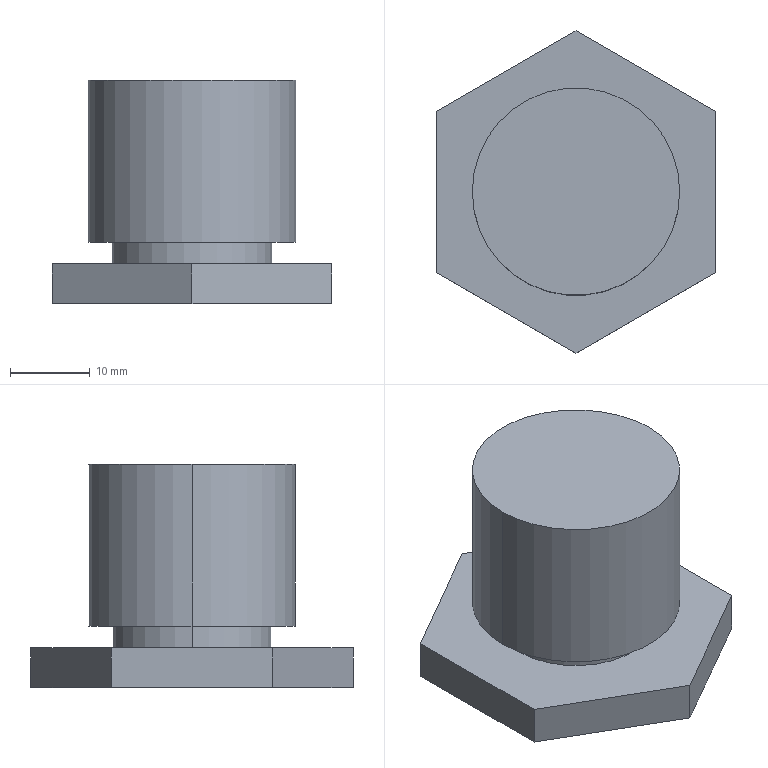Part | STEP file | Powder part sealing screw SGN-2-24 | 1 solid | 14 faces | box 35 x 40.415 x 28 mm | volume 16930 mm3 | plane 10 | cylinder 4 | commonest cylinder face diameters 20 x2 26 x2
STEP:
#1=CARTESIAN_POINT('',(0.,0.,0.));
#2=DIRECTION('',(0.,0.,1.));
#3=DIRECTION('',(1.,0.,0.));
#4=AXIS2_PLACEMENT_3D('',#1,#2,#3);
#5=CARTESIAN_POINT('',(13.,0.,23.));
#6=VERTEX_POINT('',#5);
#7=CARTESIAN_POINT('',(-13.,0.,23.));
#8=VERTEX_POINT('',#7);
#9=CARTESIAN_POINT('',(0.,0.,23.));
#10=DIRECTION('',(0.,0.,1.));
#11=DIRECTION('',(1.,0.,0.));
#12=AXIS2_PLACEMENT_3D('',#9,#10,#11);
#13=CIRCLE('',#12,13.);
#14=CARTESIAN_POINT('',(0.,0.,23.));
#15=DIRECTION('',(0.,0.,-1.));
#16=DIRECTION('',(-1.,0.,0.));
#17=AXIS2_PLACEMENT_3D('',#14,#15,#16);
#18=CYLINDRICAL_SURFACE('',#17,13.);
#19=CARTESIAN_POINT('',(3.142,0.));
#20=DIRECTION('',(-1.,0.));
#21=VECTOR('',#20,1.);
#22=LINE('',#19,#21);
#23=(GEOMETRIC_REPRESENTATION_CONTEXT(2)PARAMETRIC_REPRESENTATION_CONTEXT()REPRESENTATION_CONTEXT('',''));
#24=DEFINITIONAL_REPRESENTATION('',(#22),#23);
#25=PCURVE('',#18,#24);
#26=CARTESIAN_POINT('',(0.,0.,23.));
#27=DIRECTION('',(0.,0.,1.));
#28=DIRECTION('',(1.,0.,0.));
#29=AXIS2_PLACEMENT_3D('',#26,#27,#28);
#30=PLANE('',#29);
#31=CARTESIAN_POINT('',(0.,0.));
#32=DIRECTION('',(1.,0.));
#33=AXIS2_PLACEMENT_2D('',#31,#32);
#34=CIRCLE('',#33,13.);
#35=(GEOMETRIC_REPRESENTATION_CONTEXT(2)PARAMETRIC_REPRESENTATION_CONTEXT()REPRESENTATION_CONTEXT('',''));
#36=DEFINITIONAL_REPRESENTATION('',(#34),#35);
#37=PCURVE('',#30,#36);
#38=SURFACE_CURVE('',#13,(#25,#37),.PCURVE_S1.);
#39=EDGE_CURVE('',#6,#8,#38,.T.);
#40=ORIENTED_EDGE('',*,*,#39,.F.);
#41=CARTESIAN_POINT('',(13.,0.,2.7));
#42=VERTEX_POINT('',#41);
#43=CARTESIAN_POINT('',(13.,0.,23.));
#44=DIRECTION('',(0.,0.,-1.));
#45=VECTOR('',#44,1.);
#46=LINE('',#43,#45);
#47=CARTESIAN_POINT('',(3.142,0.));
#48=DIRECTION('',(0.,1.));
#49=VECTOR('',#48,1.);
#50=LINE('',#47,#49);
#51=(GEOMETRIC_REPRESENTATION_CONTEXT(2)PARAMETRIC_REPRESENTATION_CONTEXT()REPRESENTATION_CONTEXT('',''));
#52=DEFINITIONAL_REPRESENTATION('',(#50),#51);
#53=PCURVE('',#18,#52);
#54=CARTESIAN_POINT('',(0.,0.,23.));
#55=DIRECTION('',(0.,0.,-1.));
#56=DIRECTION('',(-1.,0.,0.));
#57=AXIS2_PLACEMENT_3D('',#54,#55,#56);
#58=CYLINDRICAL_SURFACE('',#57,13.);
#59=CARTESIAN_POINT('',(3.142,0.));
#60=DIRECTION('',(0.,1.));
#61=VECTOR('',#60,1.);
#62=LINE('',#59,#61);
#63=(GEOMETRIC_REPRESENTATION_CONTEXT(2)PARAMETRIC_REPRESENTATION_CONTEXT()REPRESENTATION_CONTEXT('',''));
#64=DEFINITIONAL_REPRESENTATION('',(#62),#63);
#65=PCURVE('',#58,#64);
#66=SURFACE_CURVE('',#46,(#53,#65),.PCURVE_S1.);
#67=EDGE_CURVE('',#6,#42,#66,.T.);
#68=ORIENTED_EDGE('',*,*,#67,.T.);
#69=CARTESIAN_POINT('',(-13.,0.,2.7));
#70=VERTEX_POINT('',#69);
#71=CARTESIAN_POINT('',(0.,0.,2.7));
#72=DIRECTION('',(0.,0.,1.));
#73=DIRECTION('',(1.,0.,0.));
#74=AXIS2_PLACEMENT_3D('',#71,#72,#73);
#75=CIRCLE('',#74,13.);
#76=CARTESIAN_POINT('',(3.142,20.3));
#77=DIRECTION('',(-1.,0.));
#78=VECTOR('',#77,1.);
#79=LINE('',#76,#78);
#80=(GEOMETRIC_REPRESENTATION_CONTEXT(2)PARAMETRIC_REPRESENTATION_CONTEXT()REPRESENTATION_CONTEXT('',''));
#81=DEFINITIONAL_REPRESENTATION('',(#79),#80);
#82=PCURVE('',#18,#81);
#83=CARTESIAN_POINT('',(0.,0.,2.7));
#84=DIRECTION('',(0.,0.,1.));
#85=DIRECTION('',(1.,0.,0.));
#86=AXIS2_PLACEMENT_3D('',#83,#84,#85);
#87=PLANE('',#86);
#88=CARTESIAN_POINT('',(0.,0.));
#89=DIRECTION('',(1.,0.));
#90=AXIS2_PLACEMENT_2D('',#88,#89);
#91=CIRCLE('',#90,13.);
#92=(GEOMETRIC_REPRESENTATION_CONTEXT(2)PARAMETRIC_REPRESENTATION_CONTEXT()REPRESENTATION_CONTEXT('',''));
#93=DEFINITIONAL_REPRESENTATION('',(#91),#92);
#94=PCURVE('',#87,#93);
#95=SURFACE_CURVE('',#75,(#82,#94),.PCURVE_S1.);
#96=EDGE_CURVE('',#42,#70,#95,.T.);
#97=ORIENTED_EDGE('',*,*,#96,.T.);
#98=CARTESIAN_POINT('',(-13.,0.,23.));
#99=DIRECTION('',(0.,0.,-1.));
#100=VECTOR('',#99,1.);
#101=LINE('',#98,#100);
#102=CARTESIAN_POINT('',(0.,0.));
#103=DIRECTION('',(0.,1.));
#104=VECTOR('',#103,1.);
#105=LINE('',#102,#104);
#106=(GEOMETRIC_REPRESENTATION_CONTEXT(2)PARAMETRIC_REPRESENTATION_CONTEXT()REPRESENTATION_CONTEXT('',''));
#107=DEFINITIONAL_REPRESENTATION('',(#105),#106);
#108=PCURVE('',#18,#107);
#109=CARTESIAN_POINT('',(6.283,0.));
#110=DIRECTION('',(0.,1.));
#111=VECTOR('',#110,1.);
#112=LINE('',#109,#111);
#113=(GEOMETRIC_REPRESENTATION_CONTEXT(2)PARAMETRIC_REPRESENTATION_CONTEXT()REPRESENTATION_CONTEXT('',''));
#114=DEFINITIONAL_REPRESENTATION('',(#112),#113);
#115=PCURVE('',#58,#114);
#116=SURFACE_CURVE('',#101,(#108,#115),.PCURVE_S1.);
#117=EDGE_CURVE('',#8,#70,#116,.T.);
#118=ORIENTED_EDGE('',*,*,#117,.F.);
#119=EDGE_LOOP('',(#40,#68,#97,#118));
#120=FACE_BOUND('',#119,.T.);
#121=ADVANCED_FACE('',(#120),#18,.T.);
#122=CARTESIAN_POINT('',(10.,0.,2.7));
#123=VERTEX_POINT('',#122);
#124=CARTESIAN_POINT('',(-10.,0.,2.7));
#125=VERTEX_POINT('',#124);
#126=CARTESIAN_POINT('',(0.,0.,2.7));
#127=DIRECTION('',(0.,0.,1.));
#128=DIRECTION('',(1.,0.,0.));
#129=AXIS2_PLACEMENT_3D('',#126,#127,#128);
#130=CIRCLE('',#129,10.);
#131=CARTESIAN_POINT('',(0.,0.,2.7));
#132=DIRECTION('',(0.,0.,-1.));
#133=DIRECTION('',(-1.,0.,0.));
#134=AXIS2_PLACEMENT_3D('',#131,#132,#133);
#135=CYLINDRICAL_SURFACE('',#134,10.);
#136=CARTESIAN_POINT('',(3.142,0.));
#137=DIRECTION('',(-1.,0.));
#138=VECTOR('',#137,1.);
#139=LINE('',#136,#138);
#140=(GEOMETRIC_REPRESENTATION_CONTEXT(2)PARAMETRIC_REPRESENTATION_CONTEXT()REPRESENTATION_CONTEXT('',''));
#141=DEFINITIONAL_REPRESENTATION('',(#139),#140);
#142=PCURVE('',#135,#141);
#143=CARTESIAN_POINT('',(0.,0.));
#144=DIRECTION('',(1.,0.));
#145=AXIS2_PLACEMENT_2D('',#143,#144);
#146=CIRCLE('',#145,10.);
#147=(GEOMETRIC_REPRESENTATION_CONTEXT(2)PARAMETRIC_REPRESENTATION_CONTEXT()REPRESENTATION_CONTEXT('',''));
#148=DEFINITIONAL_REPRESENTATION('',(#146),#147);
#149=PCURVE('',#87,#148);
#150=SURFACE_CURVE('',#130,(#142,#149),.PCURVE_S1.);
#151=EDGE_CURVE('',#123,#125,#150,.T.);
#152=ORIENTED_EDGE('',*,*,#151,.F.);
#153=CARTESIAN_POINT('',(10.,0.,0.));
#154=VERTEX_POINT('',#153);
#155=CARTESIAN_POINT('',(10.,0.,2.7));
#156=DIRECTION('',(0.,0.,-1.));
#157=VECTOR('',#156,1.);
#158=LINE('',#155,#157);
#159=CARTESIAN_POINT('',(3.142,0.));
#160=DIRECTION('',(0.,1.));
#161=VECTOR('',#160,1.);
#162=LINE('',#159,#161);
#163=(GEOMETRIC_REPRESENTATION_CONTEXT(2)PARAMETRIC_REPRESENTATION_CONTEXT()REPRESENTATION_CONTEXT('',''));
#164=DEFINITIONAL_REPRESENTATION('',(#162),#163);
#165=PCURVE('',#135,#164);
#166=CARTESIAN_POINT('',(0.,0.,2.7));
#167=DIRECTION('',(0.,0.,-1.));
#168=DIRECTION('',(-1.,0.,0.));
#169=AXIS2_PLACEMENT_3D('',#166,#167,#168);
#170=CYLINDRICAL_SURFACE('',#169,10.);
#171=CARTESIAN_POINT('',(3.142,0.));
#172=DIRECTION('',(0.,1.));
#173=VECTOR('',#172,1.);
#174=LINE('',#171,#173);
#175=(GEOMETRIC_REPRESENTATION_CONTEXT(2)PARAMETRIC_REPRESENTATION_CONTEXT()REPRESENTATION_CONTEXT('',''));
#176=DEFINITIONAL_REPRESENTATION('',(#174),#175);
#177=PCURVE('',#170,#176);
#178=SURFACE_CURVE('',#158,(#165,#177),.PCURVE_S1.);
#179=EDGE_CURVE('',#123,#154,#178,.T.);
#180=ORIENTED_EDGE('',*,*,#179,.T.);
#181=CARTESIAN_POINT('',(-10.,0.,0.));
#182=VERTEX_POINT('',#181);
#183=CARTESIAN_POINT('',(0.,0.,0.));
#184=DIRECTION('',(0.,0.,1.));
#185=DIRECTION('',(1.,0.,0.));
#186=AXIS2_PLACEMENT_3D('',#183,#184,#185);
#187=CIRCLE('',#186,10.);
#188=CARTESIAN_POINT('',(3.142,2.7));
#189=DIRECTION('',(-1.,0.));
#190=VECTOR('',#189,1.);
#191=LINE('',#188,#190);
#192=(GEOMETRIC_REPRESENTATION_CONTEXT(2)PARAMETRIC_REPRESENTATION_CONTEXT()REPRESENTATION_CONTEXT('',''));
#193=DEFINITIONAL_REPRESENTATION('',(#191),#192);
#194=PCURVE('',#135,#193);
#195=CARTESIAN_POINT('',(0.,0.,0.));
#196=DIRECTION('',(0.,0.,-1.));
#197=DIRECTION('',(-1.,0.,0.));
#198=AXIS2_PLACEMENT_3D('',#195,#196,#197);
#199=PLANE('',#198);
#200=CARTESIAN_POINT('',(-10.,0.));
#201=CARTESIAN_POINT('',(-10.,17.321));
#202=CARTESIAN_POINT('',(5.,8.66));
#203=CARTESIAN_POINT('',(20.,0.));
#204=CARTESIAN_POINT('',(5.,-8.66));
#205=CARTESIAN_POINT('',(-10.,-17.321));
#206=CARTESIAN_POINT('',(-10.,0.));
#207=(BOUNDED_CURVE()B_SPLINE_CURVE(2,(#200,#201,#202,#203,#204,#205,#206),.UNSPECIFIED.,.T.,.F.)B_SPLINE_CURVE_WITH_KNOTS((1,2,2,2,2,1),(-2.094,0.,2.094,4.189,6.283,8.378),.UNSPECIFIED.)CURVE()GEOMETRIC_REPRESENTATION_ITEM()RATIONAL_B_SPLINE_CURVE((1.,0.5,1.,0.5,1.,0.5,1.))REPRESENTATION_ITEM(''));
#208=(GEOMETRIC_REPRESENTATION_CONTEXT(2)PARAMETRIC_REPRESENTATION_CONTEXT()REPRESENTATION_CONTEXT('',''));
#209=DEFINITIONAL_REPRESENTATION('',(#207),#208);
#210=PCURVE('',#199,#209);
#211=SURFACE_CURVE('',#187,(#194,#210),.PCURVE_S1.);
#212=EDGE_CURVE('',#154,#182,#211,.T.);
#213=ORIENTED_EDGE('',*,*,#212,.T.);
#214=CARTESIAN_POINT('',(-10.,0.,2.7));
#215=DIRECTION('',(0.,0.,-1.));
#216=VECTOR('',#215,1.);
#217=LINE('',#214,#216);
#218=CARTESIAN_POINT('',(0.,0.));
#219=DIRECTION('',(0.,1.));
#220=VECTOR('',#219,1.);
#221=LINE('',#218,#220);
#222=(GEOMETRIC_REPRESENTATION_CONTEXT(2)PARAMETRIC_REPRESENTATION_CONTEXT()REPRESENTATION_CONTEXT('',''));
#223=DEFINITIONAL_REPRESENTATION('',(#221),#222);
#224=PCURVE('',#135,#223);
#225=CARTESIAN_POINT('',(6.283,0.));
#226=DIRECTION('',(0.,1.));
#227=VECTOR('',#226,1.);
#228=LINE('',#225,#227);
#229=(GEOMETRIC_REPRESENTATION_CONTEXT(2)PARAMETRIC_REPRESENTATION_CONTEXT()REPRESENTATION_CONTEXT('',''));
#230=DEFINITIONAL_REPRESENTATION('',(#228),#229);
#231=PCURVE('',#170,#230);
#232=SURFACE_CURVE('',#217,(#224,#231),.PCURVE_S1.);
#233=EDGE_CURVE('',#125,#182,#232,.T.);
#234=ORIENTED_EDGE('',*,*,#233,.F.);
#235=EDGE_LOOP('',(#152,#180,#213,#234));
#236=FACE_BOUND('',#235,.T.);
#237=ADVANCED_FACE('',(#236),#135,.T.);
#238=CARTESIAN_POINT('',(-17.5,10.104,0.));
#239=VERTEX_POINT('',#238);
#240=CARTESIAN_POINT('',(0.,20.207,0.));
#241=VERTEX_POINT('',#240);
#242=CARTESIAN_POINT('',(-17.5,10.104,0.));
#243=DIRECTION('',(0.866,0.5,0.));
#244=VECTOR('',#243,1.);
#245=LINE('',#242,#244);
#246=CARTESIAN_POINT('',(-17.5,10.104,-5.));
#247=DIRECTION('',(0.5,-0.866,0.));
#248=DIRECTION('',(0.866,0.5,0.));
#249=AXIS2_PLACEMENT_3D('',#246,#247,#248);
#250=PLANE('',#249);
#251=CARTESIAN_POINT('',(0.,5.));
#252=DIRECTION('',(1.,0.));
#253=VECTOR('',#252,1.);
#254=LINE('',#251,#253);
#255=(GEOMETRIC_REPRESENTATION_CONTEXT(2)PARAMETRIC_REPRESENTATION_CONTEXT()REPRESENTATION_CONTEXT('',''));
#256=DEFINITIONAL_REPRESENTATION('',(#254),#255);
#257=PCURVE('',#250,#256);
#258=CARTESIAN_POINT('',(17.5,10.104));
#259=DIRECTION('',(-0.866,0.5));
#260=VECTOR('',#259,1.);
#261=LINE('',#258,#260);
#262=(GEOMETRIC_REPRESENTATION_CONTEXT(2)PARAMETRIC_REPRESENTATION_CONTEXT()REPRESENTATION_CONTEXT('',''));
#263=DEFINITIONAL_REPRESENTATION('',(#261),#262);
#264=PCURVE('',#199,#263);
#265=SURFACE_CURVE('',#245,(#257,#264),.PCURVE_S1.);
#266=EDGE_CURVE('',#239,#241,#265,.T.);
#267=ORIENTED_EDGE('',*,*,#266,.T.);
#268=CARTESIAN_POINT('',(0.,20.207,-5.));
#269=VERTEX_POINT('',#268);
#270=CARTESIAN_POINT('',(0.,20.207,-5.));
#271=DIRECTION('',(0.,0.,1.));
#272=VECTOR('',#271,1.);
#273=LINE('',#270,#272);
#274=CARTESIAN_POINT('',(20.207,0.));
#275=DIRECTION('',(0.,1.));
#276=VECTOR('',#275,1.);
#277=LINE('',#274,#276);
#278=(GEOMETRIC_REPRESENTATION_CONTEXT(2)PARAMETRIC_REPRESENTATION_CONTEXT()REPRESENTATION_CONTEXT('',''));
#279=DEFINITIONAL_REPRESENTATION('',(#277),#278);
#280=PCURVE('',#250,#279);
#281=CARTESIAN_POINT('',(0.,20.207,-5.));
#282=DIRECTION('',(-0.5,-0.866,0.));
#283=DIRECTION('',(0.866,-0.5,0.));
#284=AXIS2_PLACEMENT_3D('',#281,#282,#283);
#285=PLANE('',#284);
#286=CARTESIAN_POINT('',(0.,0.));
#287=DIRECTION('',(0.,1.));
#288=VECTOR('',#287,1.);
#289=LINE('',#286,#288);
#290=(GEOMETRIC_REPRESENTATION_CONTEXT(2)PARAMETRIC_REPRESENTATION_CONTEXT()REPRESENTATION_CONTEXT('',''));
#291=DEFINITIONAL_REPRESENTATION('',(#289),#290);
#292=PCURVE('',#285,#291);
#293=SURFACE_CURVE('',#273,(#280,#292),.PCURVE_S1.);
#294=EDGE_CURVE('',#269,#241,#293,.T.);
#295=ORIENTED_EDGE('',*,*,#294,.F.);
#296=CARTESIAN_POINT('',(-17.5,10.104,-5.));
#297=VERTEX_POINT('',#296);
#298=CARTESIAN_POINT('',(-17.5,10.104,-5.));
#299=DIRECTION('',(0.866,0.5,0.));
#300=VECTOR('',#299,1.);
#301=LINE('',#298,#300);
#302=CARTESIAN_POINT('',(0.,0.));
#303=DIRECTION('',(1.,0.));
#304=VECTOR('',#303,1.);
#305=LINE('',#302,#304);
#306=(GEOMETRIC_REPRESENTATION_CONTEXT(2)PARAMETRIC_REPRESENTATION_CONTEXT()REPRESENTATION_CONTEXT('',''));
#307=DEFINITIONAL_REPRESENTATION('',(#305),#306);
#308=PCURVE('',#250,#307);
#309=CARTESIAN_POINT('',(0.,0.,-5.));
#310=DIRECTION('',(0.,0.,-1.));
#311=DIRECTION('',(-1.,0.,0.));
#312=AXIS2_PLACEMENT_3D('',#309,#310,#311);
#313=PLANE('',#312);
#314=CARTESIAN_POINT('',(17.5,10.104));
#315=DIRECTION('',(-0.866,0.5));
#316=VECTOR('',#315,1.);
#317=LINE('',#314,#316);
#318=(GEOMETRIC_REPRESENTATION_CONTEXT(2)PARAMETRIC_REPRESENTATION_CONTEXT()REPRESENTATION_CONTEXT('',''));
#319=DEFINITIONAL_REPRESENTATION('',(#317),#318);
#320=PCURVE('',#313,#319);
#321=SURFACE_CURVE('',#301,(#308,#320),.PCURVE_S1.);
#322=EDGE_CURVE('',#297,#269,#321,.T.);
#323=ORIENTED_EDGE('',*,*,#322,.F.);
#324=CARTESIAN_POINT('',(-17.5,10.104,-5.));
#325=DIRECTION('',(0.,0.,1.));
#326=VECTOR('',#325,1.);
#327=LINE('',#324,#326);
#328=CARTESIAN_POINT('',(0.,0.));
#329=DIRECTION('',(0.,1.));
#330=VECTOR('',#329,1.);
#331=LINE('',#328,#330);
#332=(GEOMETRIC_REPRESENTATION_CONTEXT(2)PARAMETRIC_REPRESENTATION_CONTEXT()REPRESENTATION_CONTEXT('',''));
#333=DEFINITIONAL_REPRESENTATION('',(#331),#332);
#334=PCURVE('',#250,#333);
#335=CARTESIAN_POINT('',(-17.5,-10.104,-5.));
#336=DIRECTION('',(1.,0.,0.));
#337=DIRECTION('',(0.,1.,0.));
#338=AXIS2_PLACEMENT_3D('',#335,#336,#337);
#339=PLANE('',#338);
#340=CARTESIAN_POINT('',(20.207,0.));
#341=DIRECTION('',(0.,1.));
#342=VECTOR('',#341,1.);
#343=LINE('',#340,#342);
#344=(GEOMETRIC_REPRESENTATION_CONTEXT(2)PARAMETRIC_REPRESENTATION_CONTEXT()REPRESENTATION_CONTEXT('',''));
#345=DEFINITIONAL_REPRESENTATION('',(#343),#344);
#346=PCURVE('',#339,#345);
#347=SURFACE_CURVE('',#327,(#334,#346),.PCURVE_S1.);
#348=EDGE_CURVE('',#297,#239,#347,.T.);
#349=ORIENTED_EDGE('',*,*,#348,.T.);
#350=EDGE_LOOP('',(#267,#295,#323,#349));
#351=FACE_BOUND('',#350,.T.);
#352=ADVANCED_FACE('',(#351),#250,.F.);
#353=CARTESIAN_POINT('',(17.5,10.104,0.));
#354=VERTEX_POINT('',#353);
#355=CARTESIAN_POINT('',(0.,20.207,0.));
#356=DIRECTION('',(0.866,-0.5,0.));
#357=VECTOR('',#356,1.);
#358=LINE('',#355,#357);
#359=CARTESIAN_POINT('',(0.,5.));
#360=DIRECTION('',(1.,0.));
#361=VECTOR('',#360,1.);
#362=LINE('',#359,#361);
#363=(GEOMETRIC_REPRESENTATION_CONTEXT(2)PARAMETRIC_REPRESENTATION_CONTEXT()REPRESENTATION_CONTEXT('',''));
#364=DEFINITIONAL_REPRESENTATION('',(#362),#363);
#365=PCURVE('',#285,#364);
#366=CARTESIAN_POINT('',(0.,20.207));
#367=DIRECTION('',(-0.866,-0.5));
#368=VECTOR('',#367,1.);
#369=LINE('',#366,#368);
#370=(GEOMETRIC_REPRESENTATION_CONTEXT(2)PARAMETRIC_REPRESENTATION_CONTEXT()REPRESENTATION_CONTEXT('',''));
#371=DEFINITIONAL_REPRESENTATION('',(#369),#370);
#372=PCURVE('',#199,#371);
#373=SURFACE_CURVE('',#358,(#365,#372),.PCURVE_S1.);
#374=EDGE_CURVE('',#241,#354,#373,.T.);
#375=ORIENTED_EDGE('',*,*,#374,.T.);
#376=CARTESIAN_POINT('',(17.5,10.104,-5.));
#377=VERTEX_POINT('',#376);
#378=CARTESIAN_POINT('',(17.5,10.104,-5.));
#379=DIRECTION('',(0.,0.,1.));
#380=VECTOR('',#379,1.);
#381=LINE('',#378,#380);
#382=CARTESIAN_POINT('',(20.207,0.));
#383=DIRECTION('',(0.,1.));
#384=VECTOR('',#383,1.);
#385=LINE('',#382,#384);
#386=(GEOMETRIC_REPRESENTATION_CONTEXT(2)PARAMETRIC_REPRESENTATION_CONTEXT()REPRESENTATION_CONTEXT('',''));
#387=DEFINITIONAL_REPRESENTATION('',(#385),#386);
#388=PCURVE('',#285,#387);
#389=CARTESIAN_POINT('',(17.5,10.104,-5.));
#390=DIRECTION('',(-1.,0.,0.));
#391=DIRECTION('',(0.,-1.,0.));
#392=AXIS2_PLACEMENT_3D('',#389,#390,#391);
#393=PLANE('',#392);
#394=CARTESIAN_POINT('',(0.,0.));
#395=DIRECTION('',(0.,1.));
#396=VECTOR('',#395,1.);
#397=LINE('',#394,#396);
#398=(GEOMETRIC_REPRESENTATION_CONTEXT(2)PARAMETRIC_REPRESENTATION_CONTEXT()REPRESENTATION_CONTEXT('',''));
#399=DEFINITIONAL_REPRESENTATION('',(#397),#398);
#400=PCURVE('',#393,#399);
#401=SURFACE_CURVE('',#381,(#388,#400),.PCURVE_S1.);
#402=EDGE_CURVE('',#377,#354,#401,.T.);
#403=ORIENTED_EDGE('',*,*,#402,.F.);
#404=CARTESIAN_POINT('',(0.,20.207,-5.));
#405=DIRECTION('',(0.866,-0.5,0.));
#406=VECTOR('',#405,1.);
#407=LINE('',#404,#406);
#408=CARTESIAN_POINT('',(0.,0.));
#409=DIRECTION('',(1.,0.));
#410=VECTOR('',#409,1.);
#411=LINE('',#408,#410);
#412=(GEOMETRIC_REPRESENTATION_CONTEXT(2)PARAMETRIC_REPRESENTATION_CONTEXT()REPRESENTATION_CONTEXT('',''));
#413=DEFINITIONAL_REPRESENTATION('',(#411),#412);
#414=PCURVE('',#285,#413);
#415=CARTESIAN_POINT('',(0.,20.207));
#416=DIRECTION('',(-0.866,-0.5));
#417=VECTOR('',#416,1.);
#418=LINE('',#415,#417);
#419=(GEOMETRIC_REPRESENTATION_CONTEXT(2)PARAMETRIC_REPRESENTATION_CONTEXT()REPRESENTATION_CONTEXT('',''));
#420=DEFINITIONAL_REPRESENTATION('',(#418),#419);
#421=PCURVE('',#313,#420);
#422=SURFACE_CURVE('',#407,(#414,#421),.PCURVE_S1.);
#423=EDGE_CURVE('',#269,#377,#422,.T.);
#424=ORIENTED_EDGE('',*,*,#423,.F.);
#425=ORIENTED_EDGE('',*,*,#294,.T.);
#426=EDGE_LOOP('',(#375,#403,#424,#425));
#427=FACE_BOUND('',#426,.T.);
#428=ADVANCED_FACE('',(#427),#285,.F.);
#429=CARTESIAN_POINT('',(17.5,-10.104,0.));
#430=VERTEX_POINT('',#429);
#431=CARTESIAN_POINT('',(17.5,10.104,0.));
#432=DIRECTION('',(0.,-1.,0.));
#433=VECTOR('',#432,1.);
#434=LINE('',#431,#433);
#435=CARTESIAN_POINT('',(0.,5.));
#436=DIRECTION('',(1.,0.));
#437=VECTOR('',#436,1.);
#438=LINE('',#435,#437);
#439=(GEOMETRIC_REPRESENTATION_CONTEXT(2)PARAMETRIC_REPRESENTATION_CONTEXT()REPRESENTATION_CONTEXT('',''));
#440=DEFINITIONAL_REPRESENTATION('',(#438),#439);
#441=PCURVE('',#393,#440);
#442=CARTESIAN_POINT('',(-17.5,10.104));
#443=DIRECTION('',(0.,-1.));
#444=VECTOR('',#443,1.);
#445=LINE('',#442,#444);
#446=(GEOMETRIC_REPRESENTATION_CONTEXT(2)PARAMETRIC_REPRESENTATION_CONTEXT()REPRESENTATION_CONTEXT('',''));
#447=DEFINITIONAL_REPRESENTATION('',(#445),#446);
#448=PCURVE('',#199,#447);
#449=SURFACE_CURVE('',#434,(#441,#448),.PCURVE_S1.);
#450=EDGE_CURVE('',#354,#430,#449,.T.);
#451=ORIENTED_EDGE('',*,*,#450,.T.);
#452=CARTESIAN_POINT('',(17.5,-10.104,-5.));
#453=VERTEX_POINT('',#452);
#454=CARTESIAN_POINT('',(17.5,-10.104,-5.));
#455=DIRECTION('',(0.,0.,1.));
#456=VECTOR('',#455,1.);
#457=LINE('',#454,#456);
#458=CARTESIAN_POINT('',(20.207,0.));
#459=DIRECTION('',(0.,1.));
#460=VECTOR('',#459,1.);
#461=LINE('',#458,#460);
#462=(GEOMETRIC_REPRESENTATION_CONTEXT(2)PARAMETRIC_REPRESENTATION_CONTEXT()REPRESENTATION_CONTEXT('',''));
#463=DEFINITIONAL_REPRESENTATION('',(#461),#462);
#464=PCURVE('',#393,#463);
#465=CARTESIAN_POINT('',(17.5,-10.104,-5.));
#466=DIRECTION('',(-0.5,0.866,0.));
#467=DIRECTION('',(-0.866,-0.5,0.));
#468=AXIS2_PLACEMENT_3D('',#465,#466,#467);
#469=PLANE('',#468);
#470=CARTESIAN_POINT('',(0.,0.));
#471=DIRECTION('',(0.,1.));
#472=VECTOR('',#471,1.);
#473=LINE('',#470,#472);
#474=(GEOMETRIC_REPRESENTATION_CONTEXT(2)PARAMETRIC_REPRESENTATION_CONTEXT()REPRESENTATION_CONTEXT('',''));
#475=DEFINITIONAL_REPRESENTATION('',(#473),#474);
#476=PCURVE('',#469,#475);
#477=SURFACE_CURVE('',#457,(#464,#476),.PCURVE_S1.);
#478=EDGE_CURVE('',#453,#430,#477,.T.);
#479=ORIENTED_EDGE('',*,*,#478,.F.);
#480=CARTESIAN_POINT('',(17.5,10.104,-5.));
#481=DIRECTION('',(0.,-1.,0.));
#482=VECTOR('',#481,1.);
#483=LINE('',#480,#482);
#484=CARTESIAN_POINT('',(0.,0.));
#485=DIRECTION('',(1.,0.));
#486=VECTOR('',#485,1.);
#487=LINE('',#484,#486);
#488=(GEOMETRIC_REPRESENTATION_CONTEXT(2)PARAMETRIC_REPRESENTATION_CONTEXT()REPRESENTATION_CONTEXT('',''));
#489=DEFINITIONAL_REPRESENTATION('',(#487),#488);
#490=PCURVE('',#393,#489);
#491=CARTESIAN_POINT('',(-17.5,10.104));
#492=DIRECTION('',(0.,-1.));
#493=VECTOR('',#492,1.);
#494=LINE('',#491,#493);
#495=(GEOMETRIC_REPRESENTATION_CONTEXT(2)PARAMETRIC_REPRESENTATION_CONTEXT()REPRESENTATION_CONTEXT('',''));
#496=DEFINITIONAL_REPRESENTATION('',(#494),#495);
#497=PCURVE('',#313,#496);
#498=SURFACE_CURVE('',#483,(#490,#497),.PCURVE_S1.);
#499=EDGE_CURVE('',#377,#453,#498,.T.);
#500=ORIENTED_EDGE('',*,*,#499,.F.);
#501=ORIENTED_EDGE('',*,*,#402,.T.);
#502=EDGE_LOOP('',(#451,#479,#500,#501));
#503=FACE_BOUND('',#502,.T.);
#504=ADVANCED_FACE('',(#503),#393,.F.);
#505=CARTESIAN_POINT('',(0.,-20.207,0.));
#506=VERTEX_POINT('',#505);
#507=CARTESIAN_POINT('',(17.5,-10.104,0.));
#508=DIRECTION('',(-0.866,-0.5,0.));
#509=VECTOR('',#508,1.);
#510=LINE('',#507,#509);
#511=CARTESIAN_POINT('',(0.,5.));
#512=DIRECTION('',(1.,0.));
#513=VECTOR('',#512,1.);
#514=LINE('',#511,#513);
#515=(GEOMETRIC_REPRESENTATION_CONTEXT(2)PARAMETRIC_REPRESENTATION_CONTEXT()REPRESENTATION_CONTEXT('',''));
#516=DEFINITIONAL_REPRESENTATION('',(#514),#515);
#517=PCURVE('',#469,#516);
#518=CARTESIAN_POINT('',(-17.5,-10.104));
#519=DIRECTION('',(0.866,-0.5));
#520=VECTOR('',#519,1.);
#521=LINE('',#518,#520);
#522=(GEOMETRIC_REPRESENTATION_CONTEXT(2)PARAMETRIC_REPRESENTATION_CONTEXT()REPRESENTATION_CONTEXT('',''));
#523=DEFINITIONAL_REPRESENTATION('',(#521),#522);
#524=PCURVE('',#199,#523);
#525=SURFACE_CURVE('',#510,(#517,#524),.PCURVE_S1.);
#526=EDGE_CURVE('',#430,#506,#525,.T.);
#527=ORIENTED_EDGE('',*,*,#526,.T.);
#528=CARTESIAN_POINT('',(0.,-20.207,-5.));
#529=VERTEX_POINT('',#528);
#530=CARTESIAN_POINT('',(0.,-20.207,-5.));
#531=DIRECTION('',(0.,0.,1.));
#532=VECTOR('',#531,1.);
#533=LINE('',#530,#532);
#534=CARTESIAN_POINT('',(20.207,0.));
#535=DIRECTION('',(0.,1.));
#536=VECTOR('',#535,1.);
#537=LINE('',#534,#536);
#538=(GEOMETRIC_REPRESENTATION_CONTEXT(2)PARAMETRIC_REPRESENTATION_CONTEXT()REPRESENTATION_CONTEXT('',''));
#539=DEFINITIONAL_REPRESENTATION('',(#537),#538);
#540=PCURVE('',#469,#539);
#541=CARTESIAN_POINT('',(0.,-20.207,-5.));
#542=DIRECTION('',(0.5,0.866,0.));
#543=DIRECTION('',(-0.866,0.5,0.));
#544=AXIS2_PLACEMENT_3D('',#541,#542,#543);
#545=PLANE('',#544);
#546=CARTESIAN_POINT('',(0.,0.));
#547=DIRECTION('',(0.,1.));
#548=VECTOR('',#547,1.);
#549=LINE('',#546,#548);
#550=(GEOMETRIC_REPRESENTATION_CONTEXT(2)PARAMETRIC_REPRESENTATION_CONTEXT()REPRESENTATION_CONTEXT('',''));
#551=DEFINITIONAL_REPRESENTATION('',(#549),#550);
#552=PCURVE('',#545,#551);
#553=SURFACE_CURVE('',#533,(#540,#552),.PCURVE_S1.);
#554=EDGE_CURVE('',#529,#506,#553,.T.);
#555=ORIENTED_EDGE('',*,*,#554,.F.);
#556=CARTESIAN_POINT('',(17.5,-10.104,-5.));
#557=DIRECTION('',(-0.866,-0.5,0.));
#558=VECTOR('',#557,1.);
#559=LINE('',#556,#558);
#560=CARTESIAN_POINT('',(0.,0.));
#561=DIRECTION('',(1.,0.));
#562=VECTOR('',#561,1.);
#563=LINE('',#560,#562);
#564=(GEOMETRIC_REPRESENTATION_CONTEXT(2)PARAMETRIC_REPRESENTATION_CONTEXT()REPRESENTATION_CONTEXT('',''));
#565=DEFINITIONAL_REPRESENTATION('',(#563),#564);
#566=PCURVE('',#469,#565);
#567=CARTESIAN_POINT('',(-17.5,-10.104));
#568=DIRECTION('',(0.866,-0.5));
#569=VECTOR('',#568,1.);
#570=LINE('',#567,#569);
#571=(GEOMETRIC_REPRESENTATION_CONTEXT(2)PARAMETRIC_REPRESENTATION_CONTEXT()REPRESENTATION_CONTEXT('',''));
#572=DEFINITIONAL_REPRESENTATION('',(#570),#571);
#573=PCURVE('',#313,#572);
#574=SURFACE_CURVE('',#559,(#566,#573),.PCURVE_S1.);
#575=EDGE_CURVE('',#453,#529,#574,.T.);
#576=ORIENTED_EDGE('',*,*,#575,.F.);
#577=ORIENTED_EDGE('',*,*,#478,.T.);
#578=EDGE_LOOP('',(#527,#555,#576,#577));
#579=FACE_BOUND('',#578,.T.);
#580=ADVANCED_FACE('',(#579),#469,.F.);
#581=CARTESIAN_POINT('',(-17.5,-10.104,0.));
#582=VERTEX_POINT('',#581);
#583=CARTESIAN_POINT('',(0.,-20.207,0.));
#584=DIRECTION('',(-0.866,0.5,0.));
#585=VECTOR('',#584,1.);
#586=LINE('',#583,#585);
#587=CARTESIAN_POINT('',(0.,5.));
#588=DIRECTION('',(1.,0.));
#589=VECTOR('',#588,1.);
#590=LINE('',#587,#589);
#591=(GEOMETRIC_REPRESENTATION_CONTEXT(2)PARAMETRIC_REPRESENTATION_CONTEXT()REPRESENTATION_CONTEXT('',''));
#592=DEFINITIONAL_REPRESENTATION('',(#590),#591);
#593=PCURVE('',#545,#592);
#594=CARTESIAN_POINT('',(0.,-20.207));
#595=DIRECTION('',(0.866,0.5));
#596=VECTOR('',#595,1.);
#597=LINE('',#594,#596);
#598=(GEOMETRIC_REPRESENTATION_CONTEXT(2)PARAMETRIC_REPRESENTATION_CONTEXT()REPRESENTATION_CONTEXT('',''));
#599=DEFINITIONAL_REPRESENTATION('',(#597),#598);
#600=PCURVE('',#199,#599);
#601=SURFACE_CURVE('',#586,(#593,#600),.PCURVE_S1.);
#602=EDGE_CURVE('',#506,#582,#601,.T.);
#603=ORIENTED_EDGE('',*,*,#602,.T.);
#604=CARTESIAN_POINT('',(-17.5,-10.104,-5.));
#605=VERTEX_POINT('',#604);
#606=CARTESIAN_POINT('',(-17.5,-10.104,-5.));
#607=DIRECTION('',(0.,0.,1.));
#608=VECTOR('',#607,1.);
#609=LINE('',#606,#608);
#610=CARTESIAN_POINT('',(20.207,0.));
#611=DIRECTION('',(0.,1.));
#612=VECTOR('',#611,1.);
#613=LINE('',#610,#612);
#614=(GEOMETRIC_REPRESENTATION_CONTEXT(2)PARAMETRIC_REPRESENTATION_CONTEXT()REPRESENTATION_CONTEXT('',''));
#615=DEFINITIONAL_REPRESENTATION('',(#613),#614);
#616=PCURVE('',#545,#615);
#617=CARTESIAN_POINT('',(0.,0.));
#618=DIRECTION('',(0.,1.));
#619=VECTOR('',#618,1.);
#620=LINE('',#617,#619);
#621=(GEOMETRIC_REPRESENTATION_CONTEXT(2)PARAMETRIC_REPRESENTATION_CONTEXT()REPRESENTATION_CONTEXT('',''));
#622=DEFINITIONAL_REPRESENTATION('',(#620),#621);
#623=PCURVE('',#339,#622);
#624=SURFACE_CURVE('',#609,(#616,#623),.PCURVE_S1.);
#625=EDGE_CURVE('',#605,#582,#624,.T.);
#626=ORIENTED_EDGE('',*,*,#625,.F.);
#627=CARTESIAN_POINT('',(0.,-20.207,-5.));
#628=DIRECTION('',(-0.866,0.5,0.));
#629=VECTOR('',#628,1.);
#630=LINE('',#627,#629);
#631=CARTESIAN_POINT('',(0.,0.));
#632=DIRECTION('',(1.,0.));
#633=VECTOR('',#632,1.);
#634=LINE('',#631,#633);
#635=(GEOMETRIC_REPRESENTATION_CONTEXT(2)PARAMETRIC_REPRESENTATION_CONTEXT()REPRESENTATION_CONTEXT('',''));
#636=DEFINITIONAL_REPRESENTATION('',(#634),#635);
#637=PCURVE('',#545,#636);
#638=CARTESIAN_POINT('',(0.,-20.207));
#639=DIRECTION('',(0.866,0.5));
#640=VECTOR('',#639,1.);
#641=LINE('',#638,#640);
#642=(GEOMETRIC_REPRESENTATION_CONTEXT(2)PARAMETRIC_REPRESENTATION_CONTEXT()REPRESENTATION_CONTEXT('',''));
#643=DEFINITIONAL_REPRESENTATION('',(#641),#642);
#644=PCURVE('',#313,#643);
#645=SURFACE_CURVE('',#630,(#637,#644),.PCURVE_S1.);
#646=EDGE_CURVE('',#529,#605,#645,.T.);
#647=ORIENTED_EDGE('',*,*,#646,.F.);
#648=ORIENTED_EDGE('',*,*,#554,.T.);
#649=EDGE_LOOP('',(#603,#626,#647,#648));
#650=FACE_BOUND('',#649,.T.);
#651=ADVANCED_FACE('',(#650),#545,.F.);
#652=CARTESIAN_POINT('',(-17.5,-10.104,0.));
#653=DIRECTION('',(0.,1.,0.));
#654=VECTOR('',#653,1.);
#655=LINE('',#652,#654);
#656=CARTESIAN_POINT('',(0.,5.));
#657=DIRECTION('',(1.,0.));
#658=VECTOR('',#657,1.);
#659=LINE('',#656,#658);
#660=(GEOMETRIC_REPRESENTATION_CONTEXT(2)PARAMETRIC_REPRESENTATION_CONTEXT()REPRESENTATION_CONTEXT('',''));
#661=DEFINITIONAL_REPRESENTATION('',(#659),#660);
#662=PCURVE('',#339,#661);
#663=CARTESIAN_POINT('',(17.5,-10.104));
#664=DIRECTION('',(0.,1.));
#665=VECTOR('',#664,1.);
#666=LINE('',#663,#665);
#667=(GEOMETRIC_REPRESENTATION_CONTEXT(2)PARAMETRIC_REPRESENTATION_CONTEXT()REPRESENTATION_CONTEXT('',''));
#668=DEFINITIONAL_REPRESENTATION('',(#666),#667);
#669=PCURVE('',#199,#668);
#670=SURFACE_CURVE('',#655,(#662,#669),.PCURVE_S1.);
#671=EDGE_CURVE('',#582,#239,#670,.T.);
#672=ORIENTED_EDGE('',*,*,#671,.T.);
#673=ORIENTED_EDGE('',*,*,#348,.F.);
#674=CARTESIAN_POINT('',(-17.5,-10.104,-5.));
#675=DIRECTION('',(0.,1.,0.));
#676=VECTOR('',#675,1.);
#677=LINE('',#674,#676);
#678=CARTESIAN_POINT('',(0.,0.));
#679=DIRECTION('',(1.,0.));
#680=VECTOR('',#679,1.);
#681=LINE('',#678,#680);
#682=(GEOMETRIC_REPRESENTATION_CONTEXT(2)PARAMETRIC_REPRESENTATION_CONTEXT()REPRESENTATION_CONTEXT('',''));
#683=DEFINITIONAL_REPRESENTATION('',(#681),#682);
#684=PCURVE('',#339,#683);
#685=CARTESIAN_POINT('',(17.5,-10.104));
#686=DIRECTION('',(0.,1.));
#687=VECTOR('',#686,1.);
#688=LINE('',#685,#687);
#689=(GEOMETRIC_REPRESENTATION_CONTEXT(2)PARAMETRIC_REPRESENTATION_CONTEXT()REPRESENTATION_CONTEXT('',''));
#690=DEFINITIONAL_REPRESENTATION('',(#688),#689);
#691=PCURVE('',#313,#690);
#692=SURFACE_CURVE('',#677,(#684,#691),.PCURVE_S1.);
#693=EDGE_CURVE('',#605,#297,#692,.T.);
#694=ORIENTED_EDGE('',*,*,#693,.F.);
#695=ORIENTED_EDGE('',*,*,#625,.T.);
#696=EDGE_LOOP('',(#672,#673,#694,#695));
#697=FACE_BOUND('',#696,.T.);
#698=ADVANCED_FACE('',(#697),#339,.F.);
#699=ORIENTED_EDGE('',*,*,#322,.T.);
#700=ORIENTED_EDGE('',*,*,#423,.T.);
#701=ORIENTED_EDGE('',*,*,#499,.T.);
#702=ORIENTED_EDGE('',*,*,#575,.T.);
#703=ORIENTED_EDGE('',*,*,#646,.T.);
#704=ORIENTED_EDGE('',*,*,#693,.T.);
#705=EDGE_LOOP('',(#699,#700,#701,#702,#703,#704));
#706=FACE_BOUND('',#705,.T.);
#707=ADVANCED_FACE('',(#706),#313,.T.);
#708=ORIENTED_EDGE('',*,*,#266,.F.);
#709=ORIENTED_EDGE('',*,*,#671,.F.);
#710=ORIENTED_EDGE('',*,*,#602,.F.);
#711=ORIENTED_EDGE('',*,*,#526,.F.);
#712=ORIENTED_EDGE('',*,*,#450,.F.);
#713=ORIENTED_EDGE('',*,*,#374,.F.);
#714=EDGE_LOOP('',(#708,#709,#710,#711,#712,#713));
#715=FACE_BOUND('',#714,.T.);
#716=CARTESIAN_POINT('',(0.,0.,0.));
#717=DIRECTION('',(0.,0.,1.));
#718=DIRECTION('',(1.,0.,0.));
#719=AXIS2_PLACEMENT_3D('',#716,#717,#718);
#720=CIRCLE('',#719,10.);
#721=CARTESIAN_POINT('',(-10.,0.));
#722=CARTESIAN_POINT('',(-10.,17.321));
#723=CARTESIAN_POINT('',(5.,8.66));
#724=CARTESIAN_POINT('',(20.,0.));
#725=CARTESIAN_POINT('',(5.,-8.66));
#726=CARTESIAN_POINT('',(-10.,-17.321));
#727=CARTESIAN_POINT('',(-10.,0.));
#728=(BOUNDED_CURVE()B_SPLINE_CURVE(2,(#721,#722,#723,#724,#725,#726,#727),.UNSPECIFIED.,.T.,.F.)B_SPLINE_CURVE_WITH_KNOTS((1,2,2,2,2,1),(-2.094,0.,2.094,4.189,6.283,8.378),.UNSPECIFIED.)CURVE()GEOMETRIC_REPRESENTATION_ITEM()RATIONAL_B_SPLINE_CURVE((1.,0.5,1.,0.5,1.,0.5,1.))REPRESENTATION_ITEM(''));
#729=(GEOMETRIC_REPRESENTATION_CONTEXT(2)PARAMETRIC_REPRESENTATION_CONTEXT()REPRESENTATION_CONTEXT('',''));
#730=DEFINITIONAL_REPRESENTATION('',(#728),#729);
#731=PCURVE('',#199,#730);
#732=CARTESIAN_POINT('',(9.425,2.7));
#733=DIRECTION('',(-1.,0.));
#734=VECTOR('',#733,1.);
#735=LINE('',#732,#734);
#736=(GEOMETRIC_REPRESENTATION_CONTEXT(2)PARAMETRIC_REPRESENTATION_CONTEXT()REPRESENTATION_CONTEXT('',''));
#737=DEFINITIONAL_REPRESENTATION('',(#735),#736);
#738=PCURVE('',#170,#737);
#739=SURFACE_CURVE('',#720,(#731,#738),.PCURVE_S1.);
#740=EDGE_CURVE('',#182,#154,#739,.T.);
#741=ORIENTED_EDGE('',*,*,#740,.F.);
#742=ORIENTED_EDGE('',*,*,#212,.F.);
#743=EDGE_LOOP('',(#741,#742));
#744=FACE_BOUND('',#743,.T.);
#745=ADVANCED_FACE('',(#715,#744),#199,.F.);
#746=CARTESIAN_POINT('',(0.,0.,2.7));
#747=DIRECTION('',(0.,0.,1.));
#748=DIRECTION('',(1.,0.,0.));
#749=AXIS2_PLACEMENT_3D('',#746,#747,#748);
#750=CIRCLE('',#749,13.);
#751=CARTESIAN_POINT('',(0.,0.));
#752=DIRECTION('',(1.,0.));
#753=AXIS2_PLACEMENT_2D('',#751,#752);
#754=CIRCLE('',#753,13.);
#755=(GEOMETRIC_REPRESENTATION_CONTEXT(2)PARAMETRIC_REPRESENTATION_CONTEXT()REPRESENTATION_CONTEXT('',''));
#756=DEFINITIONAL_REPRESENTATION('',(#754),#755);
#757=PCURVE('',#87,#756);
#758=CARTESIAN_POINT('',(9.425,20.3));
#759=DIRECTION('',(-1.,0.));
#760=VECTOR('',#759,1.);
#761=LINE('',#758,#760);
#762=(GEOMETRIC_REPRESENTATION_CONTEXT(2)PARAMETRIC_REPRESENTATION_CONTEXT()REPRESENTATION_CONTEXT('',''));
#763=DEFINITIONAL_REPRESENTATION('',(#761),#762);
#764=PCURVE('',#58,#763);
#765=SURFACE_CURVE('',#750,(#757,#764),.PCURVE_S1.);
#766=EDGE_CURVE('',#70,#42,#765,.T.);
#767=ORIENTED_EDGE('',*,*,#766,.F.);
#768=ORIENTED_EDGE('',*,*,#96,.F.);
#769=EDGE_LOOP('',(#767,#768));
#770=FACE_BOUND('',#769,.T.);
#771=CARTESIAN_POINT('',(0.,0.,2.7));
#772=DIRECTION('',(0.,0.,1.));
#773=DIRECTION('',(1.,0.,0.));
#774=AXIS2_PLACEMENT_3D('',#771,#772,#773);
#775=CIRCLE('',#774,10.);
#776=CARTESIAN_POINT('',(0.,0.));
#777=DIRECTION('',(1.,0.));
#778=AXIS2_PLACEMENT_2D('',#776,#777);
#779=CIRCLE('',#778,10.);
#780=(GEOMETRIC_REPRESENTATION_CONTEXT(2)PARAMETRIC_REPRESENTATION_CONTEXT()REPRESENTATION_CONTEXT('',''));
#781=DEFINITIONAL_REPRESENTATION('',(#779),#780);
#782=PCURVE('',#87,#781);
#783=CARTESIAN_POINT('',(9.425,0.));
#784=DIRECTION('',(-1.,0.));
#785=VECTOR('',#784,1.);
#786=LINE('',#783,#785);
#787=(GEOMETRIC_REPRESENTATION_CONTEXT(2)PARAMETRIC_REPRESENTATION_CONTEXT()REPRESENTATION_CONTEXT('',''));
#788=DEFINITIONAL_REPRESENTATION('',(#786),#787);
#789=PCURVE('',#170,#788);
#790=SURFACE_CURVE('',#775,(#782,#789),.PCURVE_S1.);
#791=EDGE_CURVE('',#125,#123,#790,.T.);
#792=ORIENTED_EDGE('',*,*,#791,.T.);
#793=ORIENTED_EDGE('',*,*,#151,.T.);
#794=EDGE_LOOP('',(#792,#793));
#795=FACE_BOUND('',#794,.T.);
#796=ADVANCED_FACE('',(#770,#795),#87,.F.);
#797=ORIENTED_EDGE('',*,*,#179,.F.);
#798=ORIENTED_EDGE('',*,*,#791,.F.);
#799=ORIENTED_EDGE('',*,*,#233,.T.);
#800=ORIENTED_EDGE('',*,*,#740,.T.);
#801=EDGE_LOOP('',(#797,#798,#799,#800));
#802=FACE_BOUND('',#801,.T.);
#803=ADVANCED_FACE('',(#802),#170,.T.);
#804=CARTESIAN_POINT('',(0.,0.,23.));
#805=DIRECTION('',(0.,0.,1.));
#806=DIRECTION('',(1.,0.,0.));
#807=AXIS2_PLACEMENT_3D('',#804,#805,#806);
#808=CIRCLE('',#807,13.);
#809=CARTESIAN_POINT('',(0.,0.));
#810=DIRECTION('',(1.,0.));
#811=AXIS2_PLACEMENT_2D('',#809,#810);
#812=CIRCLE('',#811,13.);
#813=(GEOMETRIC_REPRESENTATION_CONTEXT(2)PARAMETRIC_REPRESENTATION_CONTEXT()REPRESENTATION_CONTEXT('',''));
#814=DEFINITIONAL_REPRESENTATION('',(#812),#813);
#815=PCURVE('',#30,#814);
#816=CARTESIAN_POINT('',(9.425,0.));
#817=DIRECTION('',(-1.,0.));
#818=VECTOR('',#817,1.);
#819=LINE('',#816,#818);
#820=(GEOMETRIC_REPRESENTATION_CONTEXT(2)PARAMETRIC_REPRESENTATION_CONTEXT()REPRESENTATION_CONTEXT('',''));
#821=DEFINITIONAL_REPRESENTATION('',(#819),#820);
#822=PCURVE('',#58,#821);
#823=SURFACE_CURVE('',#808,(#815,#822),.PCURVE_S1.);
#824=EDGE_CURVE('',#8,#6,#823,.T.);
#825=ORIENTED_EDGE('',*,*,#824,.T.);
#826=ORIENTED_EDGE('',*,*,#39,.T.);
#827=EDGE_LOOP('',(#825,#826));
#828=FACE_BOUND('',#827,.T.);
#829=ADVANCED_FACE('',(#828),#30,.T.);
#830=ORIENTED_EDGE('',*,*,#67,.F.);
#831=ORIENTED_EDGE('',*,*,#824,.F.);
#832=ORIENTED_EDGE('',*,*,#117,.T.);
#833=ORIENTED_EDGE('',*,*,#766,.T.);
#834=EDGE_LOOP('',(#830,#831,#832,#833));
#835=FACE_BOUND('',#834,.T.);
#836=ADVANCED_FACE('',(#835),#58,.T.);
#837=CLOSED_SHELL('',(#121,#237,#352,#428,#504,#580,#651,#698,#707,#745,#796,#803,#829,#836));
#838=MANIFOLD_SOLID_BREP('',#837);
#839=(LENGTH_UNIT()NAMED_UNIT(*)SI_UNIT(.MILLI.,.METRE.));
#840=UNCERTAINTY_MEASURE_WITH_UNIT(LENGTH_MEASURE(0.0000001),#839,'','');
#841=(NAMED_UNIT(*)PLANE_ANGLE_UNIT()SI_UNIT($,.RADIAN.));
#842=(NAMED_UNIT(*)SI_UNIT($,.STERADIAN.)SOLID_ANGLE_UNIT());
#843=(GEOMETRIC_REPRESENTATION_CONTEXT(3)GLOBAL_UNCERTAINTY_ASSIGNED_CONTEXT((#840))GLOBAL_UNIT_ASSIGNED_CONTEXT((#839,#841,#842))REPRESENTATION_CONTEXT('',''));
#844=ADVANCED_BREP_SHAPE_REPRESENTATION('',(#4,#838),#843);